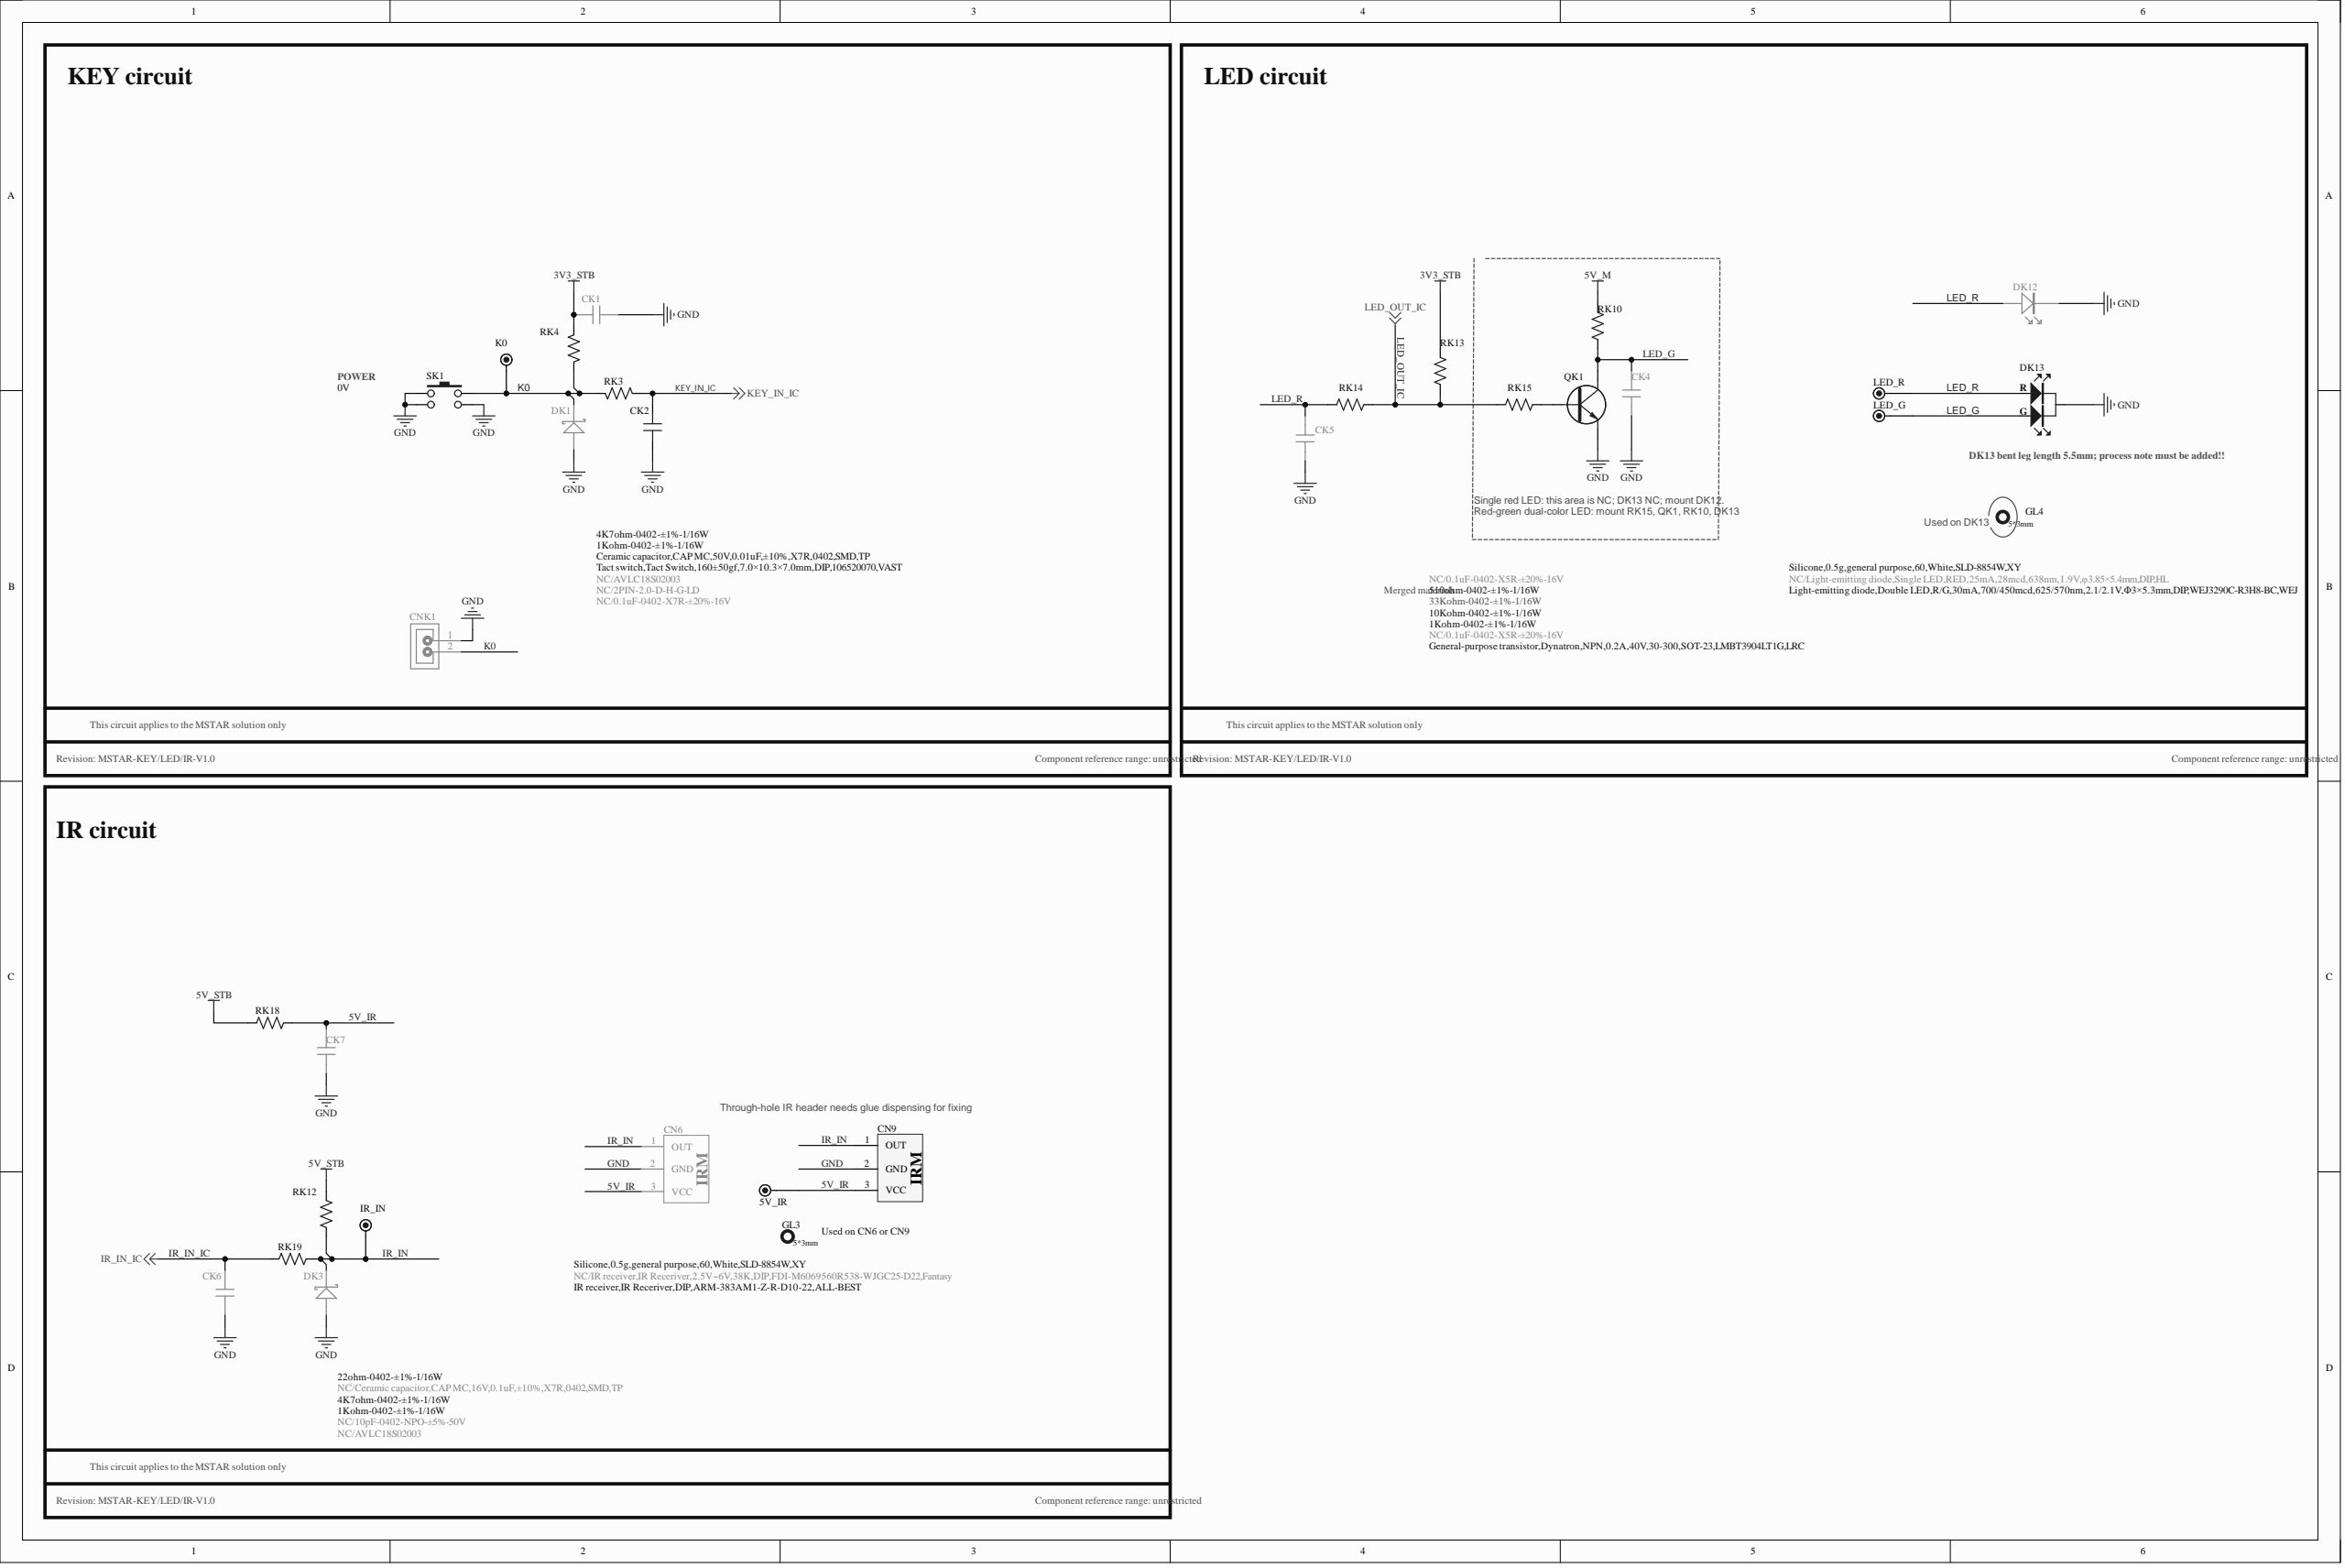Circuit board | Altium Designer | 527 parts | 243 nets | one sheet of the schematic
Parts on this sheet (reference | value | footprint):
5V_IR | TEST  SL | TP
CK1 | NC/0.1uF-0402-X7R-±20%-16V | C0402
CK2 | Ceramic capacitor,CAP MC,50V,0.01uF,±10%,X7R,0402,SMD,TP | C0402
CK4 | NC/0.1uF-0402-X5R-±20%-16V | C0402
CK5 | NC/0.1uF-0402-X5R-±20%-16V | C0402
CK6 | NC/10pF-0402-NPO-±5%-50V | C0402
CK7 | NC/Ceramic capacitor,CAP MC,16V,0.1uF,±10%,X7R,0402,SMD,TP | C0402
CN6 | NC/IR receiver,IR Receriver,2.5V~6V,38K,DIP,FDI-M6069560R538-WJGC25-D22,Fantasy | REMOTE-VD-9
CN9 | IR receiver,IR Receriver,DIP,ARM-383AM1-Z-R-D10-22,ALL-BEST | REMOTE-VD-6
CNK1 | NC/2PIN-2.0-D-H-G-LD | SIP2/2.0D-1
DK1 | NC/AVLC18S02003 | DIODE-S0402
DK3 | NC/AVLC18S02003 | DIODE-S0402
DK12 | NC/Light-emitting diode,Single LED,RED,25mA,28mcd,638nm,1.9V,f3.85×5.4mm,DIP,HL | LED-HD-6
DK13 | Light-emitting diode,Double LED,R/G,30mA,700/450mcd,625/570nm,2.1/2.1V,F3×5.3mm,DIP,WEJ3290C-R3H8-BC,WEJ | LED-HD-5
GL3 | Silicone,0.5g,general purpose,60,White,SLD-8854W,XY | Silica gel-5*3
GL4 | Silicone,0.5g,general purpose,60,White,SLD-8854W,XY | Silica gel-5*3
IR_IN | TEST  SL | TP
K0 | TEST  SL | TP
LED_G | TEST  SL | TP
LED_R | TEST  SL | TP
QK1 | General-purpose transistor,Dynatron,NPN,0.2A,40V,30-300,SOT-23,LMBT3904LT1G,LRC | SOT-23
RK3 | 1Kohm-0402-±1%-1/16W | R0402
RK4 | 4K7ohm-0402-±1%-1/16W | R0402
RK10 | 1Kohm-0402-±1%-1/16W | R0402
RK12 | 4K7ohm-0402-±1%-1/16W | R0402
RK13 | 33Kohm-0402-±1%-1/16W | R0402
RK14 | 510ohm-0402-±1%-1/16W | R0402
RK15 | 10Kohm-0402-±1%-1/16W | R0402
RK18 | 22ohm-0402-±1%-1/16W | R0402
RK19 | 1Kohm-0402-±1%-1/16W | R0402
SK1 | Tact switch,Tact Switch,160±50gf,7.0×10.3×7.0mm,DIP,106520070,VAST | KEY-HD-6
Nets of these parts (net: part-pin ...):
NetQK1_B: QK1-B RK15-1
LED_R: CK5-1 DK12-A DK13-3 LED_R-1 RK14-2
LED_OUT_IC: RK13-1 RK14-1 RK15-2
LED_G: CK4-1 DK13-1 LED_G-1 QK1-C RK10-1
KEY_IN_IC: CK2-1 RK3-1
K0: CNK1-2 DK1-K K0-1 RK3-2 RK4-1 SK1-2
IR_IN_IC: CK6-2 RK19-2
IR_IN: CN6-1 CN9-1 DK3-K IR_IN-1 RK12-1 RK19-1
GND: CK1-1 CK2-2 CK4-2 CK5-2 CK6-1 CK7-2 CN6-2 CN9-2 CNK1-1 DK1-A DK3-A DK12-K DK13-2 QK1-E SK1-1 SK1-3 SK1-4
5V_STB: RK12-2 RK18-2
5V_M: RK10-2
5V_IR: 5V_IR-1 CK7-1 CN6-3 CN9-3 RK18-1
3V3_STB: CK1-2 RK4-2 RK13-2